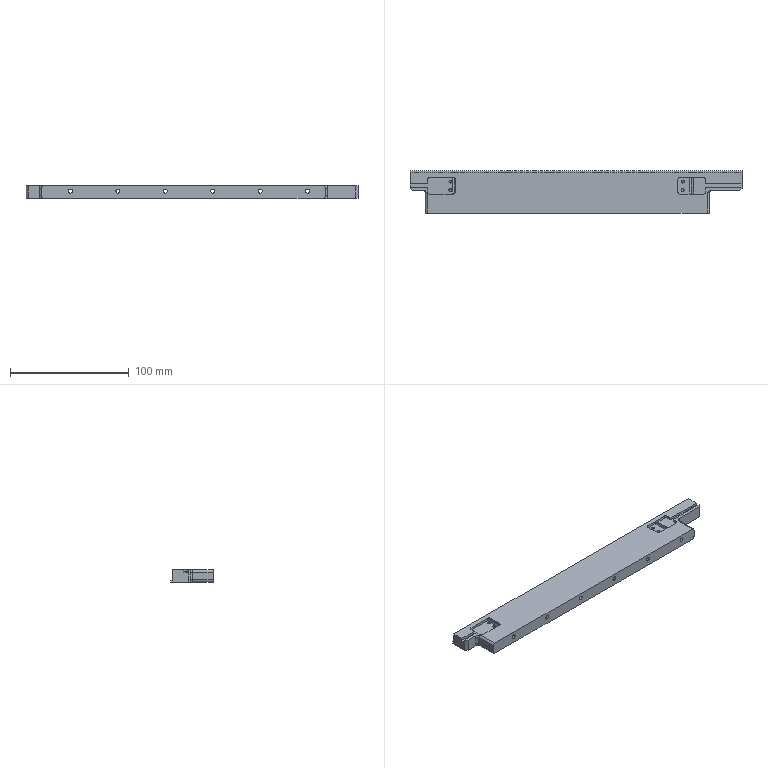Part | NX | features BREP 1 | 1 solid | 185 faces | box 280 x 35.5 x 10.5 mm | volume 85190 mm3 | cylinder 91 | cone 52 | plane 38 | torus 4 | commonest cylinder face diameters 2.5 x53 3.4 x12 6 x12 3 x8 4 x6